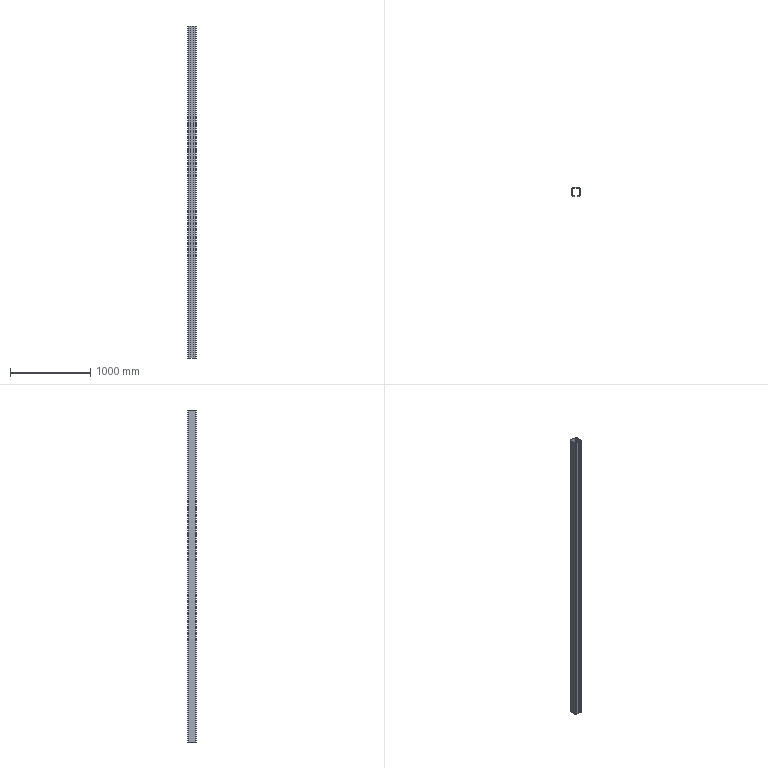Part | SolidWorks | features Extrusion 1 | 1 solid | 22 faces | box 100 x 110 x 4135 mm | volume 4470850 mm3 | plane 14 | cylinder 8 | commonest cylinder face diameters 14 x4 20 x4
STEP:
#1=CARTESIAN_POINT('',(40.,55.,0.));
#2=VERTEX_POINT('',#1);
#3=CARTESIAN_POINT('',(-40.,55.,0.));
#4=VERTEX_POINT('',#3);
#5=CARTESIAN_POINT('',(-40.,55.,0.));
#6=DIRECTION('',(-1.,0.,0.));
#7=VECTOR('',#6,1000.);
#8=LINE('',#5,#7);
#9=EDGE_CURVE('',#2,#4,#8,.T.);
#10=ORIENTED_EDGE('',*,*,#9,.T.);
#11=CARTESIAN_POINT('',(-40.,55.,4135.));
#12=VERTEX_POINT('',#11);
#13=CARTESIAN_POINT('',(-40.,55.,4135.));
#14=DIRECTION('',(0.,0.,-1.));
#15=VECTOR('',#14,1000.);
#16=LINE('',#13,#15);
#17=EDGE_CURVE('',#12,#4,#16,.T.);
#18=ORIENTED_EDGE('',*,*,#17,.F.);
#19=CARTESIAN_POINT('',(40.,55.,4135.));
#20=VERTEX_POINT('',#19);
#21=CARTESIAN_POINT('',(0.,55.,4135.));
#22=DIRECTION('',(-1.,0.,0.));
#23=VECTOR('',#22,1000.);
#24=LINE('',#21,#23);
#25=EDGE_CURVE('',#20,#12,#24,.T.);
#26=ORIENTED_EDGE('',*,*,#25,.F.);
#27=CARTESIAN_POINT('',(40.,55.,4135.));
#28=DIRECTION('',(0.,0.,-1.));
#29=VECTOR('',#28,1000.);
#30=LINE('',#27,#29);
#31=EDGE_CURVE('',#20,#2,#30,.T.);
#32=ORIENTED_EDGE('',*,*,#31,.T.);
#33=EDGE_LOOP('',(#10,#18,#26,#32));
#34=FACE_OUTER_BOUND('',#33,.T.);
#35=CARTESIAN_POINT('',(-40.,55.,4135.));
#36=DIRECTION('',(0.,-1.,0.));
#37=DIRECTION('',(0.,0.,-1.));
#38=AXIS2_PLACEMENT_3D('',#35,#36,#37);
#39=PLANE('',#38);
#40=ADVANCED_FACE('',(#34),#39,.F.);
#41=CARTESIAN_POINT('',(-50.,45.,0.));
#42=VERTEX_POINT('',#41);
#43=CARTESIAN_POINT('',(-40.,45.,0.));
#44=DIRECTION('',(0.,0.,1.));
#45=DIRECTION('',(1.,0.,0.));
#46=AXIS2_PLACEMENT_3D('',#43,#44,#45);
#47=CIRCLE('',#46,10.);
#48=EDGE_CURVE('',#4,#42,#47,.T.);
#49=ORIENTED_EDGE('',*,*,#48,.T.);
#50=CARTESIAN_POINT('',(-50.,45.,4135.));
#51=VERTEX_POINT('',#50);
#52=CARTESIAN_POINT('',(-50.,45.,4135.));
#53=DIRECTION('',(0.,0.,-1.));
#54=VECTOR('',#53,1000.);
#55=LINE('',#52,#54);
#56=EDGE_CURVE('',#51,#42,#55,.T.);
#57=ORIENTED_EDGE('',*,*,#56,.F.);
#58=CARTESIAN_POINT('',(-40.,45.,4135.));
#59=DIRECTION('',(0.,0.,1.));
#60=DIRECTION('',(1.,0.,0.));
#61=AXIS2_PLACEMENT_3D('',#58,#59,#60);
#62=CIRCLE('',#61,10.);
#63=EDGE_CURVE('',#12,#51,#62,.T.);
#64=ORIENTED_EDGE('',*,*,#63,.F.);
#65=ORIENTED_EDGE('',*,*,#17,.T.);
#66=EDGE_LOOP('',(#49,#57,#64,#65));
#67=FACE_OUTER_BOUND('',#66,.T.);
#68=CARTESIAN_POINT('',(-40.,45.,4135.));
#69=DIRECTION('',(0.,0.,-1.));
#70=DIRECTION('',(-1.,0.,0.));
#71=AXIS2_PLACEMENT_3D('',#68,#69,#70);
#72=CYLINDRICAL_SURFACE('',#71,10.);
#73=ADVANCED_FACE('',(#67),#72,.T.);
#74=CARTESIAN_POINT('',(-50.,-45.,0.));
#75=VERTEX_POINT('',#74);
#76=CARTESIAN_POINT('',(-50.,45.,0.));
#77=DIRECTION('',(0.,-1.,0.));
#78=VECTOR('',#77,1000.);
#79=LINE('',#76,#78);
#80=EDGE_CURVE('',#42,#75,#79,.T.);
#81=ORIENTED_EDGE('',*,*,#80,.T.);
#82=CARTESIAN_POINT('',(-50.,-45.,4135.));
#83=VERTEX_POINT('',#82);
#84=CARTESIAN_POINT('',(-50.,-45.,4135.));
#85=DIRECTION('',(0.,0.,-1.));
#86=VECTOR('',#85,1000.);
#87=LINE('',#84,#86);
#88=EDGE_CURVE('',#83,#75,#87,.T.);
#89=ORIENTED_EDGE('',*,*,#88,.F.);
#90=CARTESIAN_POINT('',(-50.,45.,4135.));
#91=DIRECTION('',(0.,-1.,0.));
#92=VECTOR('',#91,1000.);
#93=LINE('',#90,#92);
#94=EDGE_CURVE('',#51,#83,#93,.T.);
#95=ORIENTED_EDGE('',*,*,#94,.F.);
#96=ORIENTED_EDGE('',*,*,#56,.T.);
#97=EDGE_LOOP('',(#81,#89,#95,#96));
#98=FACE_OUTER_BOUND('',#97,.T.);
#99=CARTESIAN_POINT('',(-50.,45.,4135.));
#100=DIRECTION('',(1.,0.,0.));
#101=DIRECTION('',(0.,0.,-1.));
#102=AXIS2_PLACEMENT_3D('',#99,#100,#101);
#103=PLANE('',#102);
#104=ADVANCED_FACE('',(#98),#103,.F.);
#105=CARTESIAN_POINT('',(-40.,-55.,0.));
#106=VERTEX_POINT('',#105);
#107=CARTESIAN_POINT('',(-40.,-45.,0.));
#108=DIRECTION('',(0.,0.,1.));
#109=DIRECTION('',(1.,0.,0.));
#110=AXIS2_PLACEMENT_3D('',#107,#108,#109);
#111=CIRCLE('',#110,10.);
#112=EDGE_CURVE('',#75,#106,#111,.T.);
#113=ORIENTED_EDGE('',*,*,#112,.T.);
#114=CARTESIAN_POINT('',(-40.,-55.,4135.));
#115=VERTEX_POINT('',#114);
#116=CARTESIAN_POINT('',(-40.,-55.,4135.));
#117=DIRECTION('',(0.,0.,-1.));
#118=VECTOR('',#117,1000.);
#119=LINE('',#116,#118);
#120=EDGE_CURVE('',#115,#106,#119,.T.);
#121=ORIENTED_EDGE('',*,*,#120,.F.);
#122=CARTESIAN_POINT('',(-40.,-45.,4135.));
#123=DIRECTION('',(0.,0.,1.));
#124=DIRECTION('',(1.,0.,0.));
#125=AXIS2_PLACEMENT_3D('',#122,#123,#124);
#126=CIRCLE('',#125,10.);
#127=EDGE_CURVE('',#83,#115,#126,.T.);
#128=ORIENTED_EDGE('',*,*,#127,.F.);
#129=ORIENTED_EDGE('',*,*,#88,.T.);
#130=EDGE_LOOP('',(#113,#121,#128,#129));
#131=FACE_OUTER_BOUND('',#130,.T.);
#132=CARTESIAN_POINT('',(-40.,-45.,4135.));
#133=DIRECTION('',(0.,0.,-1.));
#134=DIRECTION('',(-1.,0.,0.));
#135=AXIS2_PLACEMENT_3D('',#132,#133,#134);
#136=CYLINDRICAL_SURFACE('',#135,10.);
#137=ADVANCED_FACE('',(#131),#136,.T.);
#138=CARTESIAN_POINT('',(-18.,-55.,0.));
#139=VERTEX_POINT('',#138);
#140=CARTESIAN_POINT('',(-40.,-55.,0.));
#141=DIRECTION('',(1.,0.,0.));
#142=VECTOR('',#141,1000.);
#143=LINE('',#140,#142);
#144=EDGE_CURVE('',#106,#139,#143,.T.);
#145=ORIENTED_EDGE('',*,*,#144,.T.);
#146=CARTESIAN_POINT('',(-18.,-55.,4135.));
#147=VERTEX_POINT('',#146);
#148=CARTESIAN_POINT('',(-18.,-55.,4135.));
#149=DIRECTION('',(0.,0.,-1.));
#150=VECTOR('',#149,1000.);
#151=LINE('',#148,#150);
#152=EDGE_CURVE('',#147,#139,#151,.T.);
#153=ORIENTED_EDGE('',*,*,#152,.F.);
#154=CARTESIAN_POINT('',(-40.,-55.,4135.));
#155=DIRECTION('',(1.,0.,0.));
#156=VECTOR('',#155,1000.);
#157=LINE('',#154,#156);
#158=EDGE_CURVE('',#115,#147,#157,.T.);
#159=ORIENTED_EDGE('',*,*,#158,.F.);
#160=ORIENTED_EDGE('',*,*,#120,.T.);
#161=EDGE_LOOP('',(#145,#153,#159,#160));
#162=FACE_OUTER_BOUND('',#161,.T.);
#163=CARTESIAN_POINT('',(-40.,-55.,4135.));
#164=DIRECTION('',(0.,1.,0.));
#165=DIRECTION('',(0.,0.,1.));
#166=AXIS2_PLACEMENT_3D('',#163,#164,#165);
#167=PLANE('',#166);
#168=ADVANCED_FACE('',(#162),#167,.F.);
#169=CARTESIAN_POINT('',(-15.,-52.,0.));
#170=VERTEX_POINT('',#169);
#171=CARTESIAN_POINT('',(-15.,-52.,0.));
#172=DIRECTION('',(0.7071,0.7071,0.));
#173=VECTOR('',#172,1000.);
#174=LINE('',#171,#173);
#175=EDGE_CURVE('',#139,#170,#174,.T.);
#176=ORIENTED_EDGE('',*,*,#175,.T.);
#177=CARTESIAN_POINT('',(-15.,-52.,4135.));
#178=VERTEX_POINT('',#177);
#179=CARTESIAN_POINT('',(-15.,-52.,4135.));
#180=DIRECTION('',(0.,0.,-1.));
#181=VECTOR('',#180,1000.);
#182=LINE('',#179,#181);
#183=EDGE_CURVE('',#178,#170,#182,.T.);
#184=ORIENTED_EDGE('',*,*,#183,.F.);
#185=CARTESIAN_POINT('',(-15.,-52.,4135.));
#186=DIRECTION('',(0.7071,0.7071,0.));
#187=VECTOR('',#186,1000.);
#188=LINE('',#185,#187);
#189=EDGE_CURVE('',#147,#178,#188,.T.);
#190=ORIENTED_EDGE('',*,*,#189,.F.);
#191=ORIENTED_EDGE('',*,*,#152,.T.);
#192=EDGE_LOOP('',(#176,#184,#190,#191));
#193=FACE_OUTER_BOUND('',#192,.T.);
#194=CARTESIAN_POINT('',(-15.,-52.,4135.));
#195=DIRECTION('',(-0.7071,0.7071,0.));
#196=DIRECTION('',(-0.7071,-0.7071,0.));
#197=AXIS2_PLACEMENT_3D('',#194,#195,#196);
#198=PLANE('',#197);
#199=ADVANCED_FACE('',(#193),#198,.F.);
#200=CARTESIAN_POINT('',(-40.,-52.,0.));
#201=VERTEX_POINT('',#200);
#202=CARTESIAN_POINT('',(-40.,-52.,0.));
#203=DIRECTION('',(-1.,0.,0.));
#204=VECTOR('',#203,1000.);
#205=LINE('',#202,#204);
#206=EDGE_CURVE('',#170,#201,#205,.T.);
#207=ORIENTED_EDGE('',*,*,#206,.T.);
#208=CARTESIAN_POINT('',(-40.,-52.,4135.));
#209=VERTEX_POINT('',#208);
#210=CARTESIAN_POINT('',(-40.,-52.,4135.));
#211=DIRECTION('',(0.,0.,-1.));
#212=VECTOR('',#211,1000.);
#213=LINE('',#210,#212);
#214=EDGE_CURVE('',#209,#201,#213,.T.);
#215=ORIENTED_EDGE('',*,*,#214,.F.);
#216=CARTESIAN_POINT('',(-40.,-52.,4135.));
#217=DIRECTION('',(-1.,0.,0.));
#218=VECTOR('',#217,1000.);
#219=LINE('',#216,#218);
#220=EDGE_CURVE('',#178,#209,#219,.T.);
#221=ORIENTED_EDGE('',*,*,#220,.F.);
#222=ORIENTED_EDGE('',*,*,#183,.T.);
#223=EDGE_LOOP('',(#207,#215,#221,#222));
#224=FACE_OUTER_BOUND('',#223,.T.);
#225=CARTESIAN_POINT('',(-40.,-52.,4135.));
#226=DIRECTION('',(0.,-1.,0.));
#227=DIRECTION('',(1.,0.,0.));
#228=AXIS2_PLACEMENT_3D('',#225,#226,#227);
#229=PLANE('',#228);
#230=ADVANCED_FACE('',(#224),#229,.F.);
#231=CARTESIAN_POINT('',(-47.,-45.,0.));
#232=VERTEX_POINT('',#231);
#233=CARTESIAN_POINT('',(-40.,-45.,0.));
#234=DIRECTION('',(0.,0.,-1.));
#235=DIRECTION('',(1.,0.,0.));
#236=AXIS2_PLACEMENT_3D('',#233,#234,#235);
#237=CIRCLE('',#236,7.);
#238=EDGE_CURVE('',#201,#232,#237,.T.);
#239=ORIENTED_EDGE('',*,*,#238,.T.);
#240=CARTESIAN_POINT('',(-47.,-45.,4135.));
#241=VERTEX_POINT('',#240);
#242=CARTESIAN_POINT('',(-47.,-45.,4135.));
#243=DIRECTION('',(0.,0.,-1.));
#244=VECTOR('',#243,1000.);
#245=LINE('',#242,#244);
#246=EDGE_CURVE('',#241,#232,#245,.T.);
#247=ORIENTED_EDGE('',*,*,#246,.F.);
#248=CARTESIAN_POINT('',(-40.,-45.,4135.));
#249=DIRECTION('',(0.,0.,-1.));
#250=DIRECTION('',(1.,0.,0.));
#251=AXIS2_PLACEMENT_3D('',#248,#249,#250);
#252=CIRCLE('',#251,7.);
#253=EDGE_CURVE('',#209,#241,#252,.T.);
#254=ORIENTED_EDGE('',*,*,#253,.F.);
#255=ORIENTED_EDGE('',*,*,#214,.T.);
#256=EDGE_LOOP('',(#239,#247,#254,#255));
#257=FACE_OUTER_BOUND('',#256,.T.);
#258=CARTESIAN_POINT('',(-40.,-45.,4135.));
#259=DIRECTION('',(0.,0.,-1.));
#260=DIRECTION('',(-1.,0.,0.));
#261=AXIS2_PLACEMENT_3D('',#258,#259,#260);
#262=CYLINDRICAL_SURFACE('',#261,7.);
#263=ADVANCED_FACE('',(#257),#262,.F.);
#264=CARTESIAN_POINT('',(-47.,45.,0.));
#265=VERTEX_POINT('',#264);
#266=CARTESIAN_POINT('',(-47.,45.,0.));
#267=DIRECTION('',(0.,1.,0.));
#268=VECTOR('',#267,1000.);
#269=LINE('',#266,#268);
#270=EDGE_CURVE('',#232,#265,#269,.T.);
#271=ORIENTED_EDGE('',*,*,#270,.T.);
#272=CARTESIAN_POINT('',(-47.,45.,4135.));
#273=VERTEX_POINT('',#272);
#274=CARTESIAN_POINT('',(-47.,45.,4135.));
#275=DIRECTION('',(0.,0.,-1.));
#276=VECTOR('',#275,1000.);
#277=LINE('',#274,#276);
#278=EDGE_CURVE('',#273,#265,#277,.T.);
#279=ORIENTED_EDGE('',*,*,#278,.F.);
#280=CARTESIAN_POINT('',(-47.,45.,4135.));
#281=DIRECTION('',(0.,1.,0.));
#282=VECTOR('',#281,1000.);
#283=LINE('',#280,#282);
#284=EDGE_CURVE('',#241,#273,#283,.T.);
#285=ORIENTED_EDGE('',*,*,#284,.F.);
#286=ORIENTED_EDGE('',*,*,#246,.T.);
#287=EDGE_LOOP('',(#271,#279,#285,#286));
#288=FACE_OUTER_BOUND('',#287,.T.);
#289=CARTESIAN_POINT('',(-47.,45.,4135.));
#290=DIRECTION('',(-1.,0.,0.));
#291=DIRECTION('',(0.,-1.,0.));
#292=AXIS2_PLACEMENT_3D('',#289,#290,#291);
#293=PLANE('',#292);
#294=ADVANCED_FACE('',(#288),#293,.F.);
#295=CARTESIAN_POINT('',(-40.,52.,0.));
#296=VERTEX_POINT('',#295);
#297=CARTESIAN_POINT('',(-40.,45.,0.));
#298=DIRECTION('',(0.,0.,-1.));
#299=DIRECTION('',(1.,0.,0.));
#300=AXIS2_PLACEMENT_3D('',#297,#298,#299);
#301=CIRCLE('',#300,7.);
#302=EDGE_CURVE('',#265,#296,#301,.T.);
#303=ORIENTED_EDGE('',*,*,#302,.T.);
#304=CARTESIAN_POINT('',(-40.,52.,4135.));
#305=VERTEX_POINT('',#304);
#306=CARTESIAN_POINT('',(-40.,52.,4135.));
#307=DIRECTION('',(0.,0.,-1.));
#308=VECTOR('',#307,1000.);
#309=LINE('',#306,#308);
#310=EDGE_CURVE('',#305,#296,#309,.T.);
#311=ORIENTED_EDGE('',*,*,#310,.F.);
#312=CARTESIAN_POINT('',(-40.,45.,4135.));
#313=DIRECTION('',(0.,0.,-1.));
#314=DIRECTION('',(1.,0.,0.));
#315=AXIS2_PLACEMENT_3D('',#312,#313,#314);
#316=CIRCLE('',#315,7.);
#317=EDGE_CURVE('',#273,#305,#316,.T.);
#318=ORIENTED_EDGE('',*,*,#317,.F.);
#319=ORIENTED_EDGE('',*,*,#278,.T.);
#320=EDGE_LOOP('',(#303,#311,#318,#319));
#321=FACE_OUTER_BOUND('',#320,.T.);
#322=CARTESIAN_POINT('',(-40.,45.,4135.));
#323=DIRECTION('',(0.,0.,-1.));
#324=DIRECTION('',(-1.,0.,0.));
#325=AXIS2_PLACEMENT_3D('',#322,#323,#324);
#326=CYLINDRICAL_SURFACE('',#325,7.);
#327=ADVANCED_FACE('',(#321),#326,.F.);
#328=CARTESIAN_POINT('',(40.,52.,0.));
#329=VERTEX_POINT('',#328);
#330=CARTESIAN_POINT('',(0.,52.,0.));
#331=DIRECTION('',(1.,0.,0.));
#332=VECTOR('',#331,1000.);
#333=LINE('',#330,#332);
#334=EDGE_CURVE('',#296,#329,#333,.T.);
#335=ORIENTED_EDGE('',*,*,#334,.T.);
#336=CARTESIAN_POINT('',(40.,52.,4135.));
#337=VERTEX_POINT('',#336);
#338=CARTESIAN_POINT('',(40.,52.,4135.));
#339=DIRECTION('',(0.,0.,-1.));
#340=VECTOR('',#339,1000.);
#341=LINE('',#338,#340);
#342=EDGE_CURVE('',#337,#329,#341,.T.);
#343=ORIENTED_EDGE('',*,*,#342,.F.);
#344=CARTESIAN_POINT('',(-40.,52.,4135.));
#345=DIRECTION('',(1.,0.,0.));
#346=VECTOR('',#345,1000.);
#347=LINE('',#344,#346);
#348=EDGE_CURVE('',#305,#337,#347,.T.);
#349=ORIENTED_EDGE('',*,*,#348,.F.);
#350=ORIENTED_EDGE('',*,*,#310,.T.);
#351=EDGE_LOOP('',(#335,#343,#349,#350));
#352=FACE_OUTER_BOUND('',#351,.T.);
#353=CARTESIAN_POINT('',(0.,52.,4135.));
#354=DIRECTION('',(0.,1.,0.));
#355=DIRECTION('',(0.,0.,1.));
#356=AXIS2_PLACEMENT_3D('',#353,#354,#355);
#357=PLANE('',#356);
#358=ADVANCED_FACE('',(#352),#357,.F.);
#359=CARTESIAN_POINT('',(47.,45.,0.));
#360=VERTEX_POINT('',#359);
#361=CARTESIAN_POINT('',(40.,45.,0.));
#362=DIRECTION('',(0.,0.,-1.));
#363=DIRECTION('',(-1.,0.,0.));
#364=AXIS2_PLACEMENT_3D('',#361,#362,#363);
#365=CIRCLE('',#364,7.);
#366=EDGE_CURVE('',#329,#360,#365,.T.);
#367=ORIENTED_EDGE('',*,*,#366,.T.);
#368=CARTESIAN_POINT('',(47.,45.,4135.));
#369=VERTEX_POINT('',#368);
#370=CARTESIAN_POINT('',(47.,45.,4135.));
#371=DIRECTION('',(0.,0.,-1.));
#372=VECTOR('',#371,1000.);
#373=LINE('',#370,#372);
#374=EDGE_CURVE('',#369,#360,#373,.T.);
#375=ORIENTED_EDGE('',*,*,#374,.F.);
#376=CARTESIAN_POINT('',(40.,45.,4135.));
#377=DIRECTION('',(0.,0.,-1.));
#378=DIRECTION('',(-1.,0.,0.));
#379=AXIS2_PLACEMENT_3D('',#376,#377,#378);
#380=CIRCLE('',#379,7.);
#381=EDGE_CURVE('',#337,#369,#380,.T.);
#382=ORIENTED_EDGE('',*,*,#381,.F.);
#383=ORIENTED_EDGE('',*,*,#342,.T.);
#384=EDGE_LOOP('',(#367,#375,#382,#383));
#385=FACE_OUTER_BOUND('',#384,.T.);
#386=CARTESIAN_POINT('',(40.,45.,4135.));
#387=DIRECTION('',(0.,0.,-1.));
#388=DIRECTION('',(-1.,0.,0.));
#389=AXIS2_PLACEMENT_3D('',#386,#387,#388);
#390=CYLINDRICAL_SURFACE('',#389,7.);
#391=ADVANCED_FACE('',(#385),#390,.F.);
#392=CARTESIAN_POINT('',(47.,-45.,0.));
#393=VERTEX_POINT('',#392);
#394=CARTESIAN_POINT('',(47.,45.,0.));
#395=DIRECTION('',(0.,-1.,0.));
#396=VECTOR('',#395,1000.);
#397=LINE('',#394,#396);
#398=EDGE_CURVE('',#360,#393,#397,.T.);
#399=ORIENTED_EDGE('',*,*,#398,.T.);
#400=CARTESIAN_POINT('',(47.,-45.,4135.));
#401=VERTEX_POINT('',#400);
#402=CARTESIAN_POINT('',(47.,-45.,4135.));
#403=DIRECTION('',(0.,0.,-1.));
#404=VECTOR('',#403,1000.);
#405=LINE('',#402,#404);
#406=EDGE_CURVE('',#401,#393,#405,.T.);
#407=ORIENTED_EDGE('',*,*,#406,.F.);
#408=CARTESIAN_POINT('',(47.,45.,4135.));
#409=DIRECTION('',(0.,-1.,0.));
#410=VECTOR('',#409,1000.);
#411=LINE('',#408,#410);
#412=EDGE_CURVE('',#369,#401,#411,.T.);
#413=ORIENTED_EDGE('',*,*,#412,.F.);
#414=ORIENTED_EDGE('',*,*,#374,.T.);
#415=EDGE_LOOP('',(#399,#407,#413,#414));
#416=FACE_OUTER_BOUND('',#415,.T.);
#417=CARTESIAN_POINT('',(47.,45.,4135.));
#418=DIRECTION('',(1.,0.,0.));
#419=DIRECTION('',(0.,1.,0.));
#420=AXIS2_PLACEMENT_3D('',#417,#418,#419);
#421=PLANE('',#420);
#422=ADVANCED_FACE('',(#416),#421,.F.);
#423=CARTESIAN_POINT('',(40.,-52.,0.));
#424=VERTEX_POINT('',#423);
#425=CARTESIAN_POINT('',(40.,-45.,0.));
#426=DIRECTION('',(0.,0.,-1.));
#427=DIRECTION('',(1.,0.,0.));
#428=AXIS2_PLACEMENT_3D('',#425,#426,#427);
#429=CIRCLE('',#428,7.);
#430=EDGE_CURVE('',#393,#424,#429,.T.);
#431=ORIENTED_EDGE('',*,*,#430,.T.);
#432=CARTESIAN_POINT('',(40.,-52.,4135.));
#433=VERTEX_POINT('',#432);
#434=CARTESIAN_POINT('',(40.,-52.,4135.));
#435=DIRECTION('',(0.,0.,-1.));
#436=VECTOR('',#435,1000.);
#437=LINE('',#434,#436);
#438=EDGE_CURVE('',#433,#424,#437,.T.);
#439=ORIENTED_EDGE('',*,*,#438,.F.);
#440=CARTESIAN_POINT('',(40.,-45.,4135.));
#441=DIRECTION('',(0.,0.,-1.));
#442=DIRECTION('',(1.,0.,0.));
#443=AXIS2_PLACEMENT_3D('',#440,#441,#442);
#444=CIRCLE('',#443,7.);
#445=EDGE_CURVE('',#401,#433,#444,.T.);
#446=ORIENTED_EDGE('',*,*,#445,.F.);
#447=ORIENTED_EDGE('',*,*,#406,.T.);
#448=EDGE_LOOP('',(#431,#439,#446,#447));
#449=FACE_OUTER_BOUND('',#448,.T.);
#450=CARTESIAN_POINT('',(40.,-45.,4135.));
#451=DIRECTION('',(0.,0.,-1.));
#452=DIRECTION('',(-1.,0.,0.));
#453=AXIS2_PLACEMENT_3D('',#450,#451,#452);
#454=CYLINDRICAL_SURFACE('',#453,7.);
#455=ADVANCED_FACE('',(#449),#454,.F.);
#456=CARTESIAN_POINT('',(15.,-52.,0.));
#457=VERTEX_POINT('',#456);
#458=CARTESIAN_POINT('',(15.,-52.,0.));
#459=DIRECTION('',(-1.,0.,0.));
#460=VECTOR('',#459,1000.);
#461=LINE('',#458,#460);
#462=EDGE_CURVE('',#424,#457,#461,.T.);
#463=ORIENTED_EDGE('',*,*,#462,.T.);
#464=CARTESIAN_POINT('',(15.,-52.,4135.));
#465=VERTEX_POINT('',#464);
#466=CARTESIAN_POINT('',(15.,-52.,4135.));
#467=DIRECTION('',(0.,0.,-1.));
#468=VECTOR('',#467,1000.);
#469=LINE('',#466,#468);
#470=EDGE_CURVE('',#465,#457,#469,.T.);
#471=ORIENTED_EDGE('',*,*,#470,.F.);
#472=CARTESIAN_POINT('',(15.,-52.,4135.));
#473=DIRECTION('',(-1.,0.,0.));
#474=VECTOR('',#473,1000.);
#475=LINE('',#472,#474);
#476=EDGE_CURVE('',#433,#465,#475,.T.);
#477=ORIENTED_EDGE('',*,*,#476,.F.);
#478=ORIENTED_EDGE('',*,*,#438,.T.);
#479=EDGE_LOOP('',(#463,#471,#477,#478));
#480=FACE_OUTER_BOUND('',#479,.T.);
#481=CARTESIAN_POINT('',(15.,-52.,4135.));
#482=DIRECTION('',(0.,-1.,0.));
#483=DIRECTION('',(0.,0.,-1.));
#484=AXIS2_PLACEMENT_3D('',#481,#482,#483);
#485=PLANE('',#484);
#486=ADVANCED_FACE('',(#480),#485,.F.);
#487=CARTESIAN_POINT('',(18.,-55.,0.));
#488=VERTEX_POINT('',#487);
#489=CARTESIAN_POINT('',(15.,-52.,0.));
#490=DIRECTION('',(0.7071,-0.7071,0.));
#491=VECTOR('',#490,1000.);
#492=LINE('',#489,#491);
#493=EDGE_CURVE('',#457,#488,#492,.T.);
#494=ORIENTED_EDGE('',*,*,#493,.T.);
#495=CARTESIAN_POINT('',(18.,-55.,4135.));
#496=VERTEX_POINT('',#495);
#497=CARTESIAN_POINT('',(18.,-55.,4135.));
#498=DIRECTION('',(0.,0.,-1.));
#499=VECTOR('',#498,1000.);
#500=LINE('',#497,#499);
#501=EDGE_CURVE('',#496,#488,#500,.T.);
#502=ORIENTED_EDGE('',*,*,#501,.F.);
#503=CARTESIAN_POINT('',(15.,-52.,4135.));
#504=DIRECTION('',(0.7071,-0.7071,0.));
#505=VECTOR('',#504,1000.);
#506=LINE('',#503,#505);
#507=EDGE_CURVE('',#465,#496,#506,.T.);
#508=ORIENTED_EDGE('',*,*,#507,.F.);
#509=ORIENTED_EDGE('',*,*,#470,.T.);
#510=EDGE_LOOP('',(#494,#502,#508,#509));
#511=FACE_OUTER_BOUND('',#510,.T.);
#512=CARTESIAN_POINT('',(15.,-52.,4135.));
#513=DIRECTION('',(0.7071,0.7071,0.));
#514=DIRECTION('',(-0.7071,0.7071,0.));
#515=AXIS2_PLACEMENT_3D('',#512,#513,#514);
#516=PLANE('',#515);
#517=ADVANCED_FACE('',(#511),#516,.F.);
#518=CARTESIAN_POINT('',(40.,-55.,0.));
#519=VERTEX_POINT('',#518);
#520=CARTESIAN_POINT('',(18.,-55.,0.));
#521=DIRECTION('',(1.,0.,0.));
#522=VECTOR('',#521,1000.);
#523=LINE('',#520,#522);
#524=EDGE_CURVE('',#488,#519,#523,.T.);
#525=ORIENTED_EDGE('',*,*,#524,.T.);
#526=CARTESIAN_POINT('',(40.,-55.,4135.));
#527=VERTEX_POINT('',#526);
#528=CARTESIAN_POINT('',(40.,-55.,4135.));
#529=DIRECTION('',(0.,0.,-1.));
#530=VECTOR('',#529,1000.);
#531=LINE('',#528,#530);
#532=EDGE_CURVE('',#527,#519,#531,.T.);
#533=ORIENTED_EDGE('',*,*,#532,.F.);
#534=CARTESIAN_POINT('',(18.,-55.,4135.));
#535=DIRECTION('',(1.,0.,0.));
#536=VECTOR('',#535,1000.);
#537=LINE('',#534,#536);
#538=EDGE_CURVE('',#496,#527,#537,.T.);
#539=ORIENTED_EDGE('',*,*,#538,.F.);
#540=ORIENTED_EDGE('',*,*,#501,.T.);
#541=EDGE_LOOP('',(#525,#533,#539,#540));
#542=FACE_OUTER_BOUND('',#541,.T.);
#543=CARTESIAN_POINT('',(18.,-55.,4135.));
#544=DIRECTION('',(0.,1.,0.));
#545=DIRECTION('',(-1.,0.,0.));
#546=AXIS2_PLACEMENT_3D('',#543,#544,#545);
#547=PLANE('',#546);
#548=ADVANCED_FACE('',(#542),#547,.F.);
#549=CARTESIAN_POINT('',(50.,-45.,0.));
#550=VERTEX_POINT('',#549);
#551=CARTESIAN_POINT('',(40.,-45.,0.));
#552=DIRECTION('',(0.,0.,1.));
#553=DIRECTION('',(1.,0.,0.));
#554=AXIS2_PLACEMENT_3D('',#551,#552,#553);
#555=CIRCLE('',#554,10.);
#556=EDGE_CURVE('',#519,#550,#555,.T.);
#557=ORIENTED_EDGE('',*,*,#556,.T.);
#558=CARTESIAN_POINT('',(50.,-45.,4135.));
#559=VERTEX_POINT('',#558);
#560=CARTESIAN_POINT('',(50.,-45.,4135.));
#561=DIRECTION('',(0.,0.,-1.));
#562=VECTOR('',#561,1000.);
#563=LINE('',#560,#562);
#564=EDGE_CURVE('',#559,#550,#563,.T.);
#565=ORIENTED_EDGE('',*,*,#564,.F.);
#566=CARTESIAN_POINT('',(40.,-45.,4135.));
#567=DIRECTION('',(0.,0.,1.));
#568=DIRECTION('',(1.,0.,0.));
#569=AXIS2_PLACEMENT_3D('',#566,#567,#568);
#570=CIRCLE('',#569,10.);
#571=EDGE_CURVE('',#527,#559,#570,.T.);
#572=ORIENTED_EDGE('',*,*,#571,.F.);
#573=ORIENTED_EDGE('',*,*,#532,.T.);
#574=EDGE_LOOP('',(#557,#565,#572,#573));
#575=FACE_OUTER_BOUND('',#574,.T.);
#576=CARTESIAN_POINT('',(40.,-45.,4135.));
#577=DIRECTION('',(0.,0.,-1.));
#578=DIRECTION('',(-1.,0.,0.));
#579=AXIS2_PLACEMENT_3D('',#576,#577,#578);
#580=CYLINDRICAL_SURFACE('',#579,10.);
#581=ADVANCED_FACE('',(#575),#580,.T.);
#582=CARTESIAN_POINT('',(50.,45.,0.));
#583=VERTEX_POINT('',#582);
#584=CARTESIAN_POINT('',(50.,45.,0.));
#585=DIRECTION('',(0.,1.,0.));
#586=VECTOR('',#585,1000.);
#587=LINE('',#584,#586);
#588=EDGE_CURVE('',#550,#583,#587,.T.);
#589=ORIENTED_EDGE('',*,*,#588,.T.);
#590=CARTESIAN_POINT('',(50.,45.,4135.));
#591=VERTEX_POINT('',#590);
#592=CARTESIAN_POINT('',(50.,45.,4135.));
#593=DIRECTION('',(0.,0.,-1.));
#594=VECTOR('',#593,1000.);
#595=LINE('',#592,#594);
#596=EDGE_CURVE('',#591,#583,#595,.T.);
#597=ORIENTED_EDGE('',*,*,#596,.F.);
#598=CARTESIAN_POINT('',(50.,45.,4135.));
#599=DIRECTION('',(0.,1.,0.));
#600=VECTOR('',#599,1000.);
#601=LINE('',#598,#600);
#602=EDGE_CURVE('',#559,#591,#601,.T.);
#603=ORIENTED_EDGE('',*,*,#602,.F.);
#604=ORIENTED_EDGE('',*,*,#564,.T.);
#605=EDGE_LOOP('',(#589,#597,#603,#604));
#606=FACE_OUTER_BOUND('',#605,.T.);
#607=CARTESIAN_POINT('',(50.,45.,4135.));
#608=DIRECTION('',(-1.,0.,0.));
#609=DIRECTION('',(0.,-1.,0.));
#610=AXIS2_PLACEMENT_3D('',#607,#608,#609);
#611=PLANE('',#610);
#612=ADVANCED_FACE('',(#606),#611,.F.);
#613=CARTESIAN_POINT('',(40.,45.,0.));
#614=DIRECTION('',(0.,0.,1.));
#615=DIRECTION('',(-1.,0.,0.));
#616=AXIS2_PLACEMENT_3D('',#613,#614,#615);
#617=CIRCLE('',#616,10.);
#618=EDGE_CURVE('',#583,#2,#617,.T.);
#619=ORIENTED_EDGE('',*,*,#618,.T.);
#620=ORIENTED_EDGE('',*,*,#31,.F.);
#621=CARTESIAN_POINT('',(40.,45.,4135.));
#622=DIRECTION('',(0.,0.,1.));
#623=DIRECTION('',(-1.,0.,0.));
#624=AXIS2_PLACEMENT_3D('',#621,#622,#623);
#625=CIRCLE('',#624,10.);
#626=EDGE_CURVE('',#591,#20,#625,.T.);
#627=ORIENTED_EDGE('',*,*,#626,.F.);
#628=ORIENTED_EDGE('',*,*,#596,.T.);
#629=EDGE_LOOP('',(#619,#620,#627,#628));
#630=FACE_OUTER_BOUND('',#629,.T.);
#631=CARTESIAN_POINT('',(40.,45.,4135.));
#632=DIRECTION('',(0.,0.,-1.));
#633=DIRECTION('',(-1.,0.,0.));
#634=AXIS2_PLACEMENT_3D('',#631,#632,#633);
#635=CYLINDRICAL_SURFACE('',#634,10.);
#636=ADVANCED_FACE('',(#630),#635,.T.);
#637=ORIENTED_EDGE('',*,*,#25,.T.);
#638=ORIENTED_EDGE('',*,*,#63,.T.);
#639=ORIENTED_EDGE('',*,*,#94,.T.);
#640=ORIENTED_EDGE('',*,*,#127,.T.);
#641=ORIENTED_EDGE('',*,*,#158,.T.);
#642=ORIENTED_EDGE('',*,*,#189,.T.);
#643=ORIENTED_EDGE('',*,*,#220,.T.);
#644=ORIENTED_EDGE('',*,*,#253,.T.);
#645=ORIENTED_EDGE('',*,*,#284,.T.);
#646=ORIENTED_EDGE('',*,*,#317,.T.);
#647=ORIENTED_EDGE('',*,*,#348,.T.);
#648=ORIENTED_EDGE('',*,*,#381,.T.);
#649=ORIENTED_EDGE('',*,*,#412,.T.);
#650=ORIENTED_EDGE('',*,*,#445,.T.);
#651=ORIENTED_EDGE('',*,*,#476,.T.);
#652=ORIENTED_EDGE('',*,*,#507,.T.);
#653=ORIENTED_EDGE('',*,*,#538,.T.);
#654=ORIENTED_EDGE('',*,*,#571,.T.);
#655=ORIENTED_EDGE('',*,*,#602,.T.);
#656=ORIENTED_EDGE('',*,*,#626,.T.);
#657=EDGE_LOOP('',(#637,#638,#639,#640,#641,#642,#643,#644,#645,#646,#647,#648,#649,#650,#651,#652,#653,#654,#655,#656));
#658=FACE_OUTER_BOUND('',#657,.T.);
#659=CARTESIAN_POINT('',(40.,45.,4135.));
#660=DIRECTION('',(0.,0.,-1.));
#661=DIRECTION('',(-1.,0.,0.));
#662=AXIS2_PLACEMENT_3D('',#659,#660,#661);
#663=PLANE('',#662);
#664=ADVANCED_FACE('',(#658),#663,.F.);
#665=ORIENTED_EDGE('',*,*,#9,.F.);
#666=ORIENTED_EDGE('',*,*,#618,.F.);
#667=ORIENTED_EDGE('',*,*,#588,.F.);
#668=ORIENTED_EDGE('',*,*,#556,.F.);
#669=ORIENTED_EDGE('',*,*,#524,.F.);
#670=ORIENTED_EDGE('',*,*,#493,.F.);
#671=ORIENTED_EDGE('',*,*,#462,.F.);
#672=ORIENTED_EDGE('',*,*,#430,.F.);
#673=ORIENTED_EDGE('',*,*,#398,.F.);
#674=ORIENTED_EDGE('',*,*,#366,.F.);
#675=ORIENTED_EDGE('',*,*,#334,.F.);
#676=ORIENTED_EDGE('',*,*,#302,.F.);
#677=ORIENTED_EDGE('',*,*,#270,.F.);
#678=ORIENTED_EDGE('',*,*,#238,.F.);
#679=ORIENTED_EDGE('',*,*,#206,.F.);
#680=ORIENTED_EDGE('',*,*,#175,.F.);
#681=ORIENTED_EDGE('',*,*,#144,.F.);
#682=ORIENTED_EDGE('',*,*,#112,.F.);
#683=ORIENTED_EDGE('',*,*,#80,.F.);
#684=ORIENTED_EDGE('',*,*,#48,.F.);
#685=EDGE_LOOP('',(#665,#666,#667,#668,#669,#670,#671,#672,#673,#674,#675,#676,#677,#678,#679,#680,#681,#682,#683,#684));
#686=FACE_OUTER_BOUND('',#685,.T.);
#687=CARTESIAN_POINT('',(40.,45.,0.));
#688=DIRECTION('',(0.,0.,-1.));
#689=DIRECTION('',(-1.,0.,0.));
#690=AXIS2_PLACEMENT_3D('',#687,#688,#689);
#691=PLANE('',#690);
#692=ADVANCED_FACE('',(#686),#691,.T.);
#693=CLOSED_SHELL('',(#40,#73,#104,#137,#168,#199,#230,#263,#294,#327,#358,#391,#422,#455,#486,#517,#548,#581,#612,#636,#664,#692));
#694=MANIFOLD_SOLID_BREP('',#693);
#695=CARTESIAN_POINT('',(0.,0.,0.));
#696=DIRECTION('',(0.,0.,1.));
#697=DIRECTION('',(1.,0.,0.));
#698=AXIS2_PLACEMENT_3D('',#695,#696,#697);
#699=(LENGTH_UNIT()NAMED_UNIT(*)SI_UNIT(.MILLI.,.METRE.));
#700=UNCERTAINTY_MEASURE_WITH_UNIT(LENGTH_MEASURE(0.00001),#699,'','');
#701=(NAMED_UNIT(*)PLANE_ANGLE_UNIT()SI_UNIT($,.RADIAN.));
#702=(NAMED_UNIT(*)SI_UNIT($,.STERADIAN.)SOLID_ANGLE_UNIT());
#703=(GEOMETRIC_REPRESENTATION_CONTEXT(3)GLOBAL_UNCERTAINTY_ASSIGNED_CONTEXT((#700))GLOBAL_UNIT_ASSIGNED_CONTEXT((#699,#701,#702))REPRESENTATION_CONTEXT('',''));
#704=ADVANCED_BREP_SHAPE_REPRESENTATION('',(#694,#698),#703);